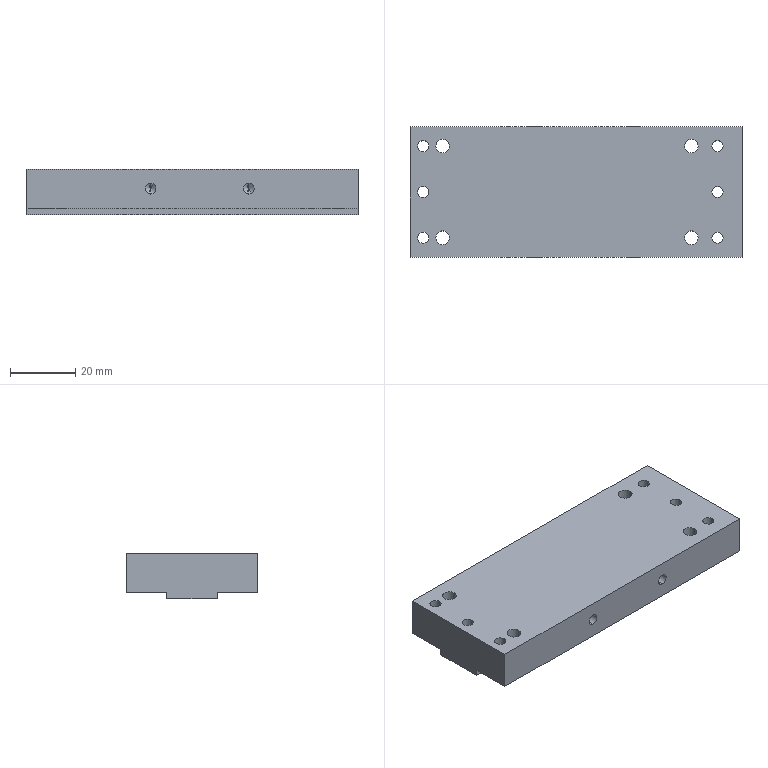Part | STEP file | track (2) | 1 solid | 64 faces | box 101.5 x 40 x 14 mm | volume 49700 mm3 | cylinder 40 | plane 16 | cone 8 | commonest cylinder face diameters 3.4 x12 6.5 x12 3.3 x8 4.2 x8